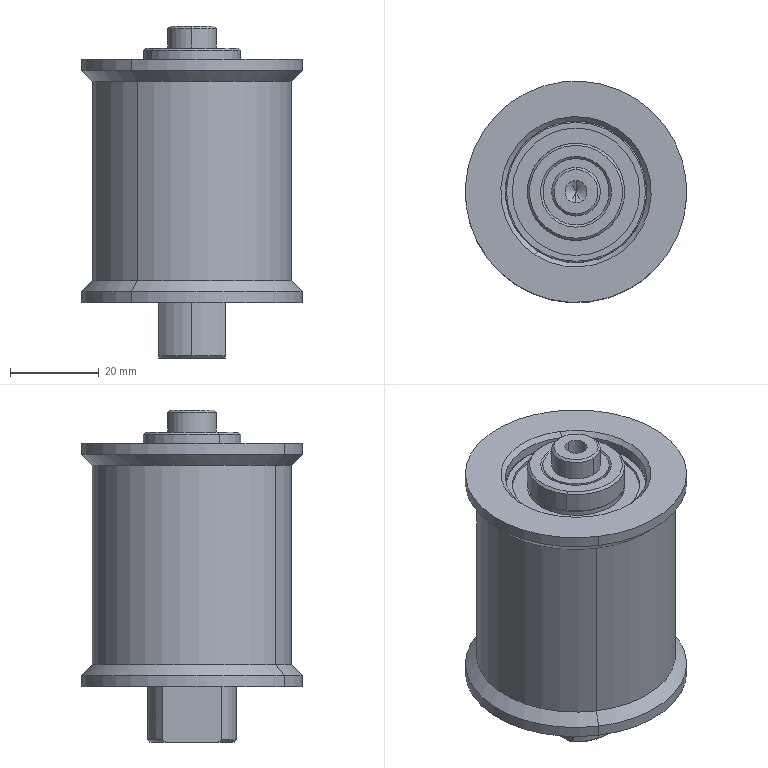Part | SolidWorks | 5 solids | 354 faces | box 50 x 50 x 75 mm | volume 77764 mm3 | sphere 108 | torus 82 | cylinder 73 | plane 65 | cone 26 | commonest cylinder face diameters 28.8 x16 15 x8 20.4 x8 21.971 x8 32 x8 23.29 x4